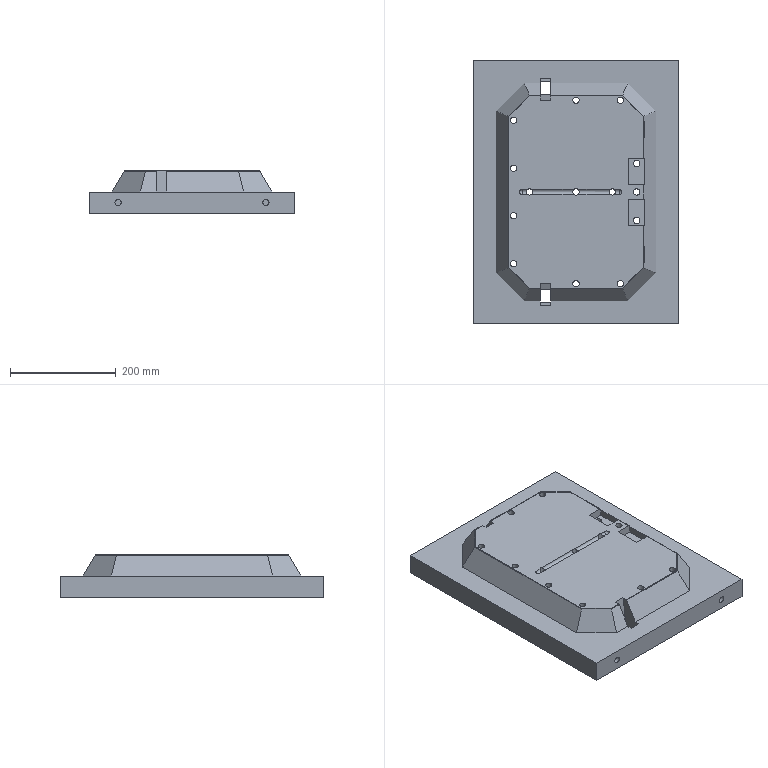Part | NX | features 模具.stp<1>[3] 2 | 1 solid | 155 faces | box 390 x 500 x 80 mm | volume 11534780 mm3 | plane 91 | cylinder 55 | cone 7 | sphere 2 | commonest cylinder face diameters 12 x32 10.5 x7 11.7 x7 10 x4 96.927 x4 13 x1